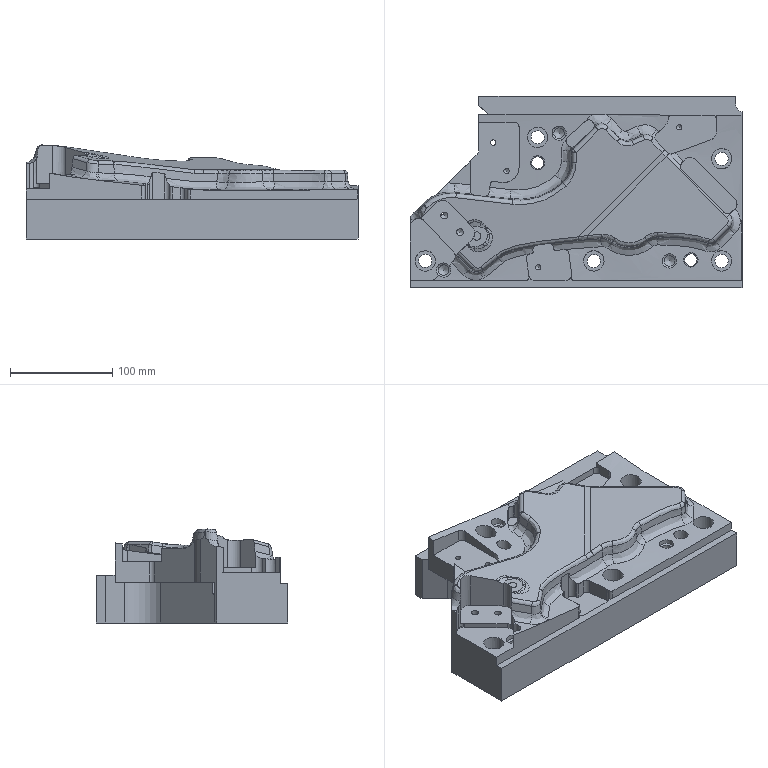Part | STEP file | gslz 2016.10.28-13_id106_x_t | 1 solid | 282 faces | box 325 x 187 x 92.051 mm | volume 3014596 mm3 | spline 112 | cylinder 76 | plane 69 | other 13 | cone 11 | sphere 1 | commonest cylinder face diameters 7.5 x9 8 x8 10 x7 14 x7 13 x5 20 x5